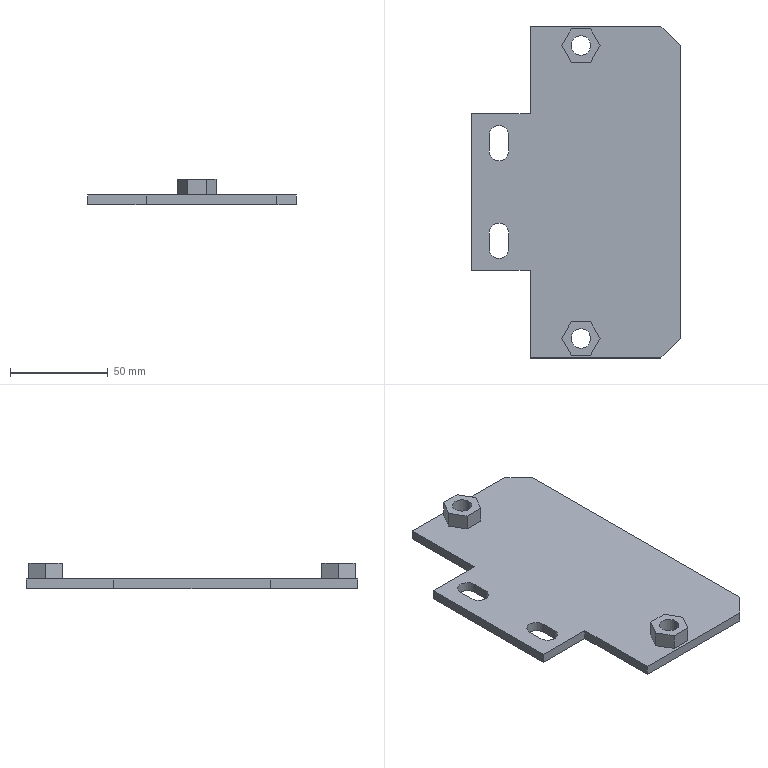Part | SolidWorks | features ICE 4, Chamfer 1, CombineBodies 1, Extrusion 1 | 3 solids | 44 faces | box 107 x 170 x 13 mm | volume 76885 mm3 | plane 32 | cylinder 12 | commonest cylinder face diameters 10 x8 12.5 x4
STEP:
#1=CARTESIAN_POINT('',(-5.,75.,13.));
#2=VERTEX_POINT('',#1);
#3=CARTESIAN_POINT('',(5.,75.,13.));
#4=VERTEX_POINT('',#3);
#5=CARTESIAN_POINT('',(0.,75.,13.));
#6=DIRECTION('',(0.,0.,1.));
#7=DIRECTION('',(1.,0.,0.));
#8=AXIS2_PLACEMENT_3D('',#5,#6,#7);
#9=CIRCLE('',#8,5.);
#10=EDGE_CURVE('',#2,#4,#9,.T.);
#11=ORIENTED_EDGE('',*,*,#10,.T.);
#12=CARTESIAN_POINT('',(5.,75.,5.));
#13=VERTEX_POINT('',#12);
#14=CARTESIAN_POINT('',(5.,75.,13.));
#15=DIRECTION('',(0.,0.,-1.));
#16=VECTOR('',#15,1000.);
#17=LINE('',#14,#16);
#18=EDGE_CURVE('',#4,#13,#17,.T.);
#19=ORIENTED_EDGE('',*,*,#18,.T.);
#20=CARTESIAN_POINT('',(-5.,75.,5.));
#21=VERTEX_POINT('',#20);
#22=CARTESIAN_POINT('',(0.,75.,5.));
#23=DIRECTION('',(0.,0.,1.));
#24=DIRECTION('',(1.,0.,0.));
#25=AXIS2_PLACEMENT_3D('',#22,#23,#24);
#26=CIRCLE('',#25,5.);
#27=EDGE_CURVE('',#21,#13,#26,.T.);
#28=ORIENTED_EDGE('',*,*,#27,.F.);
#29=CARTESIAN_POINT('',(-5.,75.,13.));
#30=DIRECTION('',(0.,0.,-1.));
#31=VECTOR('',#30,1000.);
#32=LINE('',#29,#31);
#33=EDGE_CURVE('',#2,#21,#32,.T.);
#34=ORIENTED_EDGE('',*,*,#33,.F.);
#35=EDGE_LOOP('',(#11,#19,#28,#34));
#36=FACE_OUTER_BOUND('',#35,.T.);
#37=CARTESIAN_POINT('',(0.,75.,13.));
#38=DIRECTION('',(0.,0.,-1.));
#39=DIRECTION('',(-1.,0.,0.));
#40=AXIS2_PLACEMENT_3D('',#37,#38,#39);
#41=CYLINDRICAL_SURFACE('',#40,5.);
#42=ADVANCED_FACE('',(#36),#41,.F.);
#43=CARTESIAN_POINT('',(4.907,66.5,13.));
#44=VERTEX_POINT('',#43);
#45=CARTESIAN_POINT('',(9.815,75.,13.));
#46=VERTEX_POINT('',#45);
#47=CARTESIAN_POINT('',(4.907,66.5,13.));
#48=DIRECTION('',(0.5,0.866,0.));
#49=VECTOR('',#48,1000.);
#50=LINE('',#47,#49);
#51=EDGE_CURVE('',#44,#46,#50,.T.);
#52=ORIENTED_EDGE('',*,*,#51,.T.);
#53=CARTESIAN_POINT('',(4.907,83.5,13.));
#54=VERTEX_POINT('',#53);
#55=CARTESIAN_POINT('',(9.815,75.,13.));
#56=DIRECTION('',(-0.5,0.866,0.));
#57=VECTOR('',#56,1000.);
#58=LINE('',#55,#57);
#59=EDGE_CURVE('',#46,#54,#58,.T.);
#60=ORIENTED_EDGE('',*,*,#59,.T.);
#61=CARTESIAN_POINT('',(-4.907,83.5,13.));
#62=VERTEX_POINT('',#61);
#63=CARTESIAN_POINT('',(4.907,83.5,13.));
#64=DIRECTION('',(-1.,0.,0.));
#65=VECTOR('',#64,1000.);
#66=LINE('',#63,#65);
#67=EDGE_CURVE('',#54,#62,#66,.T.);
#68=ORIENTED_EDGE('',*,*,#67,.T.);
#69=CARTESIAN_POINT('',(-9.815,75.,13.));
#70=VERTEX_POINT('',#69);
#71=CARTESIAN_POINT('',(-4.907,83.5,13.));
#72=DIRECTION('',(-0.5,-0.866,0.));
#73=VECTOR('',#72,1000.);
#74=LINE('',#71,#73);
#75=EDGE_CURVE('',#62,#70,#74,.T.);
#76=ORIENTED_EDGE('',*,*,#75,.T.);
#77=CARTESIAN_POINT('',(-4.907,66.5,13.));
#78=VERTEX_POINT('',#77);
#79=CARTESIAN_POINT('',(-9.815,75.,13.));
#80=DIRECTION('',(0.5,-0.866,0.));
#81=VECTOR('',#80,1000.);
#82=LINE('',#79,#81);
#83=EDGE_CURVE('',#70,#78,#82,.T.);
#84=ORIENTED_EDGE('',*,*,#83,.T.);
#85=CARTESIAN_POINT('',(-4.907,66.5,13.));
#86=DIRECTION('',(1.,0.,0.));
#87=VECTOR('',#86,1000.);
#88=LINE('',#85,#87);
#89=EDGE_CURVE('',#78,#44,#88,.T.);
#90=ORIENTED_EDGE('',*,*,#89,.T.);
#91=EDGE_LOOP('',(#52,#60,#68,#76,#84,#90));
#92=FACE_OUTER_BOUND('',#91,.T.);
#93=ORIENTED_EDGE('',*,*,#10,.F.);
#94=CARTESIAN_POINT('',(0.,75.,13.));
#95=DIRECTION('',(0.,0.,1.));
#96=DIRECTION('',(1.,0.,0.));
#97=AXIS2_PLACEMENT_3D('',#94,#95,#96);
#98=CIRCLE('',#97,5.);
#99=EDGE_CURVE('',#4,#2,#98,.T.);
#100=ORIENTED_EDGE('',*,*,#99,.F.);
#101=EDGE_LOOP('',(#93,#100));
#102=FACE_BOUND('',#101,.T.);
#103=CARTESIAN_POINT('',(0.,0.,13.));
#104=DIRECTION('',(0.,0.,1.));
#105=DIRECTION('',(1.,0.,0.));
#106=AXIS2_PLACEMENT_3D('',#103,#104,#105);
#107=PLANE('',#106);
#108=ADVANCED_FACE('',(#92,#102),#107,.T.);
#109=CARTESIAN_POINT('',(4.907,66.5,5.));
#110=VERTEX_POINT('',#109);
#111=CARTESIAN_POINT('',(9.815,75.,5.));
#112=VERTEX_POINT('',#111);
#113=CARTESIAN_POINT('',(4.907,66.5,5.));
#114=DIRECTION('',(0.5,0.866,0.));
#115=VECTOR('',#114,1000.);
#116=LINE('',#113,#115);
#117=EDGE_CURVE('',#110,#112,#116,.T.);
#118=ORIENTED_EDGE('',*,*,#117,.F.);
#119=CARTESIAN_POINT('',(-4.907,66.5,5.));
#120=VERTEX_POINT('',#119);
#121=CARTESIAN_POINT('',(-4.907,66.5,5.));
#122=DIRECTION('',(1.,0.,0.));
#123=VECTOR('',#122,1000.);
#124=LINE('',#121,#123);
#125=EDGE_CURVE('',#120,#110,#124,.T.);
#126=ORIENTED_EDGE('',*,*,#125,.F.);
#127=CARTESIAN_POINT('',(-9.815,75.,5.));
#128=VERTEX_POINT('',#127);
#129=CARTESIAN_POINT('',(-9.815,75.,5.));
#130=DIRECTION('',(0.5,-0.866,0.));
#131=VECTOR('',#130,1000.);
#132=LINE('',#129,#131);
#133=EDGE_CURVE('',#128,#120,#132,.T.);
#134=ORIENTED_EDGE('',*,*,#133,.F.);
#135=CARTESIAN_POINT('',(-4.907,83.5,5.));
#136=VERTEX_POINT('',#135);
#137=CARTESIAN_POINT('',(-4.907,83.5,5.));
#138=DIRECTION('',(-0.5,-0.866,0.));
#139=VECTOR('',#138,1000.);
#140=LINE('',#137,#139);
#141=EDGE_CURVE('',#136,#128,#140,.T.);
#142=ORIENTED_EDGE('',*,*,#141,.F.);
#143=CARTESIAN_POINT('',(4.907,83.5,5.));
#144=VERTEX_POINT('',#143);
#145=CARTESIAN_POINT('',(4.907,83.5,5.));
#146=DIRECTION('',(-1.,0.,0.));
#147=VECTOR('',#146,1000.);
#148=LINE('',#145,#147);
#149=EDGE_CURVE('',#144,#136,#148,.T.);
#150=ORIENTED_EDGE('',*,*,#149,.F.);
#151=CARTESIAN_POINT('',(9.815,75.,5.));
#152=DIRECTION('',(-0.5,0.866,0.));
#153=VECTOR('',#152,1000.);
#154=LINE('',#151,#153);
#155=EDGE_CURVE('',#112,#144,#154,.T.);
#156=ORIENTED_EDGE('',*,*,#155,.F.);
#157=EDGE_LOOP('',(#118,#126,#134,#142,#150,#156));
#158=FACE_OUTER_BOUND('',#157,.T.);
#159=ORIENTED_EDGE('',*,*,#27,.T.);
#160=CARTESIAN_POINT('',(0.,75.,5.));
#161=DIRECTION('',(0.,0.,1.));
#162=DIRECTION('',(1.,0.,0.));
#163=AXIS2_PLACEMENT_3D('',#160,#161,#162);
#164=CIRCLE('',#163,5.);
#165=EDGE_CURVE('',#13,#21,#164,.T.);
#166=ORIENTED_EDGE('',*,*,#165,.T.);
#167=EDGE_LOOP('',(#159,#166));
#168=FACE_BOUND('',#167,.T.);
#169=CARTESIAN_POINT('',(0.,0.,5.));
#170=DIRECTION('',(0.,0.,1.));
#171=DIRECTION('',(1.,0.,0.));
#172=AXIS2_PLACEMENT_3D('',#169,#170,#171);
#173=PLANE('',#172);
#174=ADVANCED_FACE('',(#158,#168),#173,.F.);
#175=ORIENTED_EDGE('',*,*,#117,.T.);
#176=CARTESIAN_POINT('',(9.815,75.,13.));
#177=DIRECTION('',(0.,0.,-1.));
#178=VECTOR('',#177,1000.);
#179=LINE('',#176,#178);
#180=EDGE_CURVE('',#46,#112,#179,.T.);
#181=ORIENTED_EDGE('',*,*,#180,.F.);
#182=ORIENTED_EDGE('',*,*,#51,.F.);
#183=CARTESIAN_POINT('',(4.907,66.5,13.));
#184=DIRECTION('',(0.,0.,-1.));
#185=VECTOR('',#184,1000.);
#186=LINE('',#183,#185);
#187=EDGE_CURVE('',#44,#110,#186,.T.);
#188=ORIENTED_EDGE('',*,*,#187,.T.);
#189=EDGE_LOOP('',(#175,#181,#182,#188));
#190=FACE_OUTER_BOUND('',#189,.T.);
#191=CARTESIAN_POINT('',(4.907,66.5,13.));
#192=DIRECTION('',(-0.866,0.5,0.));
#193=DIRECTION('',(-0.5,-0.866,0.));
#194=AXIS2_PLACEMENT_3D('',#191,#192,#193);
#195=PLANE('',#194);
#196=ADVANCED_FACE('',(#190),#195,.F.);
#197=ORIENTED_EDGE('',*,*,#155,.T.);
#198=CARTESIAN_POINT('',(4.907,83.5,13.));
#199=DIRECTION('',(0.,0.,-1.));
#200=VECTOR('',#199,1000.);
#201=LINE('',#198,#200);
#202=EDGE_CURVE('',#54,#144,#201,.T.);
#203=ORIENTED_EDGE('',*,*,#202,.F.);
#204=ORIENTED_EDGE('',*,*,#59,.F.);
#205=ORIENTED_EDGE('',*,*,#180,.T.);
#206=EDGE_LOOP('',(#197,#203,#204,#205));
#207=FACE_OUTER_BOUND('',#206,.T.);
#208=CARTESIAN_POINT('',(9.815,75.,13.));
#209=DIRECTION('',(-0.866,-0.5,0.));
#210=DIRECTION('',(0.5,-0.866,0.));
#211=AXIS2_PLACEMENT_3D('',#208,#209,#210);
#212=PLANE('',#211);
#213=ADVANCED_FACE('',(#207),#212,.F.);
#214=ORIENTED_EDGE('',*,*,#149,.T.);
#215=CARTESIAN_POINT('',(-4.907,83.5,13.));
#216=DIRECTION('',(0.,0.,-1.));
#217=VECTOR('',#216,1000.);
#218=LINE('',#215,#217);
#219=EDGE_CURVE('',#62,#136,#218,.T.);
#220=ORIENTED_EDGE('',*,*,#219,.F.);
#221=ORIENTED_EDGE('',*,*,#67,.F.);
#222=ORIENTED_EDGE('',*,*,#202,.T.);
#223=EDGE_LOOP('',(#214,#220,#221,#222));
#224=FACE_OUTER_BOUND('',#223,.T.);
#225=CARTESIAN_POINT('',(4.907,83.5,13.));
#226=DIRECTION('',(0.,-1.,0.));
#227=DIRECTION('',(0.,0.,-1.));
#228=AXIS2_PLACEMENT_3D('',#225,#226,#227);
#229=PLANE('',#228);
#230=ADVANCED_FACE('',(#224),#229,.F.);
#231=ORIENTED_EDGE('',*,*,#141,.T.);
#232=CARTESIAN_POINT('',(-9.815,75.,13.));
#233=DIRECTION('',(0.,0.,-1.));
#234=VECTOR('',#233,1000.);
#235=LINE('',#232,#234);
#236=EDGE_CURVE('',#70,#128,#235,.T.);
#237=ORIENTED_EDGE('',*,*,#236,.F.);
#238=ORIENTED_EDGE('',*,*,#75,.F.);
#239=ORIENTED_EDGE('',*,*,#219,.T.);
#240=EDGE_LOOP('',(#231,#237,#238,#239));
#241=FACE_OUTER_BOUND('',#240,.T.);
#242=CARTESIAN_POINT('',(-4.907,83.5,13.));
#243=DIRECTION('',(0.866,-0.5,0.));
#244=DIRECTION('',(0.5,0.866,0.));
#245=AXIS2_PLACEMENT_3D('',#242,#243,#244);
#246=PLANE('',#245);
#247=ADVANCED_FACE('',(#241),#246,.F.);
#248=ORIENTED_EDGE('',*,*,#133,.T.);
#249=CARTESIAN_POINT('',(-4.907,66.5,13.));
#250=DIRECTION('',(0.,0.,-1.));
#251=VECTOR('',#250,1000.);
#252=LINE('',#249,#251);
#253=EDGE_CURVE('',#78,#120,#252,.T.);
#254=ORIENTED_EDGE('',*,*,#253,.F.);
#255=ORIENTED_EDGE('',*,*,#83,.F.);
#256=ORIENTED_EDGE('',*,*,#236,.T.);
#257=EDGE_LOOP('',(#248,#254,#255,#256));
#258=FACE_OUTER_BOUND('',#257,.T.);
#259=CARTESIAN_POINT('',(-9.815,75.,13.));
#260=DIRECTION('',(0.866,0.5,0.));
#261=DIRECTION('',(-0.5,0.866,0.));
#262=AXIS2_PLACEMENT_3D('',#259,#260,#261);
#263=PLANE('',#262);
#264=ADVANCED_FACE('',(#258),#263,.F.);
#265=ORIENTED_EDGE('',*,*,#125,.T.);
#266=ORIENTED_EDGE('',*,*,#187,.F.);
#267=ORIENTED_EDGE('',*,*,#89,.F.);
#268=ORIENTED_EDGE('',*,*,#253,.T.);
#269=EDGE_LOOP('',(#265,#266,#267,#268));
#270=FACE_OUTER_BOUND('',#269,.T.);
#271=CARTESIAN_POINT('',(-4.907,66.5,13.));
#272=DIRECTION('',(0.,1.,0.));
#273=DIRECTION('',(-1.,0.,0.));
#274=AXIS2_PLACEMENT_3D('',#271,#272,#273);
#275=PLANE('',#274);
#276=ADVANCED_FACE('',(#270),#275,.F.);
#277=ORIENTED_EDGE('',*,*,#18,.F.);
#278=ORIENTED_EDGE('',*,*,#99,.T.);
#279=ORIENTED_EDGE('',*,*,#33,.T.);
#280=ORIENTED_EDGE('',*,*,#165,.F.);
#281=EDGE_LOOP('',(#277,#278,#279,#280));
#282=FACE_OUTER_BOUND('',#281,.T.);
#283=CARTESIAN_POINT('',(0.,75.,13.));
#284=DIRECTION('',(0.,0.,-1.));
#285=DIRECTION('',(-1.,0.,0.));
#286=AXIS2_PLACEMENT_3D('',#283,#284,#285);
#287=CYLINDRICAL_SURFACE('',#286,5.);
#288=ADVANCED_FACE('',(#282),#287,.F.);
#289=CLOSED_SHELL('',(#42,#108,#174,#196,#213,#230,#247,#264,#276,#288));
#290=MANIFOLD_SOLID_BREP('',#289);
#291=CARTESIAN_POINT('',(-5.,-75.,13.));
#292=VERTEX_POINT('',#291);
#293=CARTESIAN_POINT('',(5.,-75.,13.));
#294=VERTEX_POINT('',#293);
#295=CARTESIAN_POINT('',(0.,-75.,13.));
#296=DIRECTION('',(0.,0.,1.));
#297=DIRECTION('',(1.,0.,0.));
#298=AXIS2_PLACEMENT_3D('',#295,#296,#297);
#299=CIRCLE('',#298,5.);
#300=EDGE_CURVE('',#292,#294,#299,.T.);
#301=ORIENTED_EDGE('',*,*,#300,.T.);
#302=CARTESIAN_POINT('',(5.,-75.,5.));
#303=VERTEX_POINT('',#302);
#304=CARTESIAN_POINT('',(5.,-75.,13.));
#305=DIRECTION('',(0.,0.,-1.));
#306=VECTOR('',#305,1000.);
#307=LINE('',#304,#306);
#308=EDGE_CURVE('',#294,#303,#307,.T.);
#309=ORIENTED_EDGE('',*,*,#308,.T.);
#310=CARTESIAN_POINT('',(-5.,-75.,5.));
#311=VERTEX_POINT('',#310);
#312=CARTESIAN_POINT('',(0.,-75.,5.));
#313=DIRECTION('',(0.,0.,1.));
#314=DIRECTION('',(1.,0.,0.));
#315=AXIS2_PLACEMENT_3D('',#312,#313,#314);
#316=CIRCLE('',#315,5.);
#317=EDGE_CURVE('',#311,#303,#316,.T.);
#318=ORIENTED_EDGE('',*,*,#317,.F.);
#319=CARTESIAN_POINT('',(-5.,-75.,13.));
#320=DIRECTION('',(0.,0.,-1.));
#321=VECTOR('',#320,1000.);
#322=LINE('',#319,#321);
#323=EDGE_CURVE('',#292,#311,#322,.T.);
#324=ORIENTED_EDGE('',*,*,#323,.F.);
#325=EDGE_LOOP('',(#301,#309,#318,#324));
#326=FACE_OUTER_BOUND('',#325,.T.);
#327=CARTESIAN_POINT('',(0.,-75.,13.));
#328=DIRECTION('',(0.,0.,-1.));
#329=DIRECTION('',(-1.,0.,0.));
#330=AXIS2_PLACEMENT_3D('',#327,#328,#329);
#331=CYLINDRICAL_SURFACE('',#330,5.);
#332=ADVANCED_FACE('',(#326),#331,.F.);
#333=CARTESIAN_POINT('',(4.907,-83.5,13.));
#334=VERTEX_POINT('',#333);
#335=CARTESIAN_POINT('',(9.815,-75.,13.));
#336=VERTEX_POINT('',#335);
#337=CARTESIAN_POINT('',(4.907,-83.5,13.));
#338=DIRECTION('',(0.5,0.866,0.));
#339=VECTOR('',#338,1000.);
#340=LINE('',#337,#339);
#341=EDGE_CURVE('',#334,#336,#340,.T.);
#342=ORIENTED_EDGE('',*,*,#341,.T.);
#343=CARTESIAN_POINT('',(4.907,-66.5,13.));
#344=VERTEX_POINT('',#343);
#345=CARTESIAN_POINT('',(9.815,-75.,13.));
#346=DIRECTION('',(-0.5,0.866,0.));
#347=VECTOR('',#346,1000.);
#348=LINE('',#345,#347);
#349=EDGE_CURVE('',#336,#344,#348,.T.);
#350=ORIENTED_EDGE('',*,*,#349,.T.);
#351=CARTESIAN_POINT('',(-4.907,-66.5,13.));
#352=VERTEX_POINT('',#351);
#353=CARTESIAN_POINT('',(4.907,-66.5,13.));
#354=DIRECTION('',(-1.,0.,0.));
#355=VECTOR('',#354,1000.);
#356=LINE('',#353,#355);
#357=EDGE_CURVE('',#344,#352,#356,.T.);
#358=ORIENTED_EDGE('',*,*,#357,.T.);
#359=CARTESIAN_POINT('',(-9.815,-75.,13.));
#360=VERTEX_POINT('',#359);
#361=CARTESIAN_POINT('',(-4.907,-66.5,13.));
#362=DIRECTION('',(-0.5,-0.866,0.));
#363=VECTOR('',#362,1000.);
#364=LINE('',#361,#363);
#365=EDGE_CURVE('',#352,#360,#364,.T.);
#366=ORIENTED_EDGE('',*,*,#365,.T.);
#367=CARTESIAN_POINT('',(-4.907,-83.5,13.));
#368=VERTEX_POINT('',#367);
#369=CARTESIAN_POINT('',(-9.815,-75.,13.));
#370=DIRECTION('',(0.5,-0.866,0.));
#371=VECTOR('',#370,1000.);
#372=LINE('',#369,#371);
#373=EDGE_CURVE('',#360,#368,#372,.T.);
#374=ORIENTED_EDGE('',*,*,#373,.T.);
#375=CARTESIAN_POINT('',(-4.907,-83.5,13.));
#376=DIRECTION('',(1.,0.,0.));
#377=VECTOR('',#376,1000.);
#378=LINE('',#375,#377);
#379=EDGE_CURVE('',#368,#334,#378,.T.);
#380=ORIENTED_EDGE('',*,*,#379,.T.);
#381=EDGE_LOOP('',(#342,#350,#358,#366,#374,#380));
#382=FACE_OUTER_BOUND('',#381,.T.);
#383=ORIENTED_EDGE('',*,*,#300,.F.);
#384=CARTESIAN_POINT('',(0.,-75.,13.));
#385=DIRECTION('',(0.,0.,1.));
#386=DIRECTION('',(1.,0.,0.));
#387=AXIS2_PLACEMENT_3D('',#384,#385,#386);
#388=CIRCLE('',#387,5.);
#389=EDGE_CURVE('',#294,#292,#388,.T.);
#390=ORIENTED_EDGE('',*,*,#389,.F.);
#391=EDGE_LOOP('',(#383,#390));
#392=FACE_BOUND('',#391,.T.);
#393=CARTESIAN_POINT('',(0.,0.,13.));
#394=DIRECTION('',(0.,0.,1.));
#395=DIRECTION('',(1.,0.,0.));
#396=AXIS2_PLACEMENT_3D('',#393,#394,#395);
#397=PLANE('',#396);
#398=ADVANCED_FACE('',(#382,#392),#397,.T.);
#399=CARTESIAN_POINT('',(4.907,-83.5,5.));
#400=VERTEX_POINT('',#399);
#401=CARTESIAN_POINT('',(9.815,-75.,5.));
#402=VERTEX_POINT('',#401);
#403=CARTESIAN_POINT('',(4.907,-83.5,5.));
#404=DIRECTION('',(0.5,0.866,0.));
#405=VECTOR('',#404,1000.);
#406=LINE('',#403,#405);
#407=EDGE_CURVE('',#400,#402,#406,.T.);
#408=ORIENTED_EDGE('',*,*,#407,.F.);
#409=CARTESIAN_POINT('',(-4.907,-83.5,5.));
#410=VERTEX_POINT('',#409);
#411=CARTESIAN_POINT('',(-4.907,-83.5,5.));
#412=DIRECTION('',(1.,0.,0.));
#413=VECTOR('',#412,1000.);
#414=LINE('',#411,#413);
#415=EDGE_CURVE('',#410,#400,#414,.T.);
#416=ORIENTED_EDGE('',*,*,#415,.F.);
#417=CARTESIAN_POINT('',(-9.815,-75.,5.));
#418=VERTEX_POINT('',#417);
#419=CARTESIAN_POINT('',(-9.815,-75.,5.));
#420=DIRECTION('',(0.5,-0.866,0.));
#421=VECTOR('',#420,1000.);
#422=LINE('',#419,#421);
#423=EDGE_CURVE('',#418,#410,#422,.T.);
#424=ORIENTED_EDGE('',*,*,#423,.F.);
#425=CARTESIAN_POINT('',(-4.907,-66.5,5.));
#426=VERTEX_POINT('',#425);
#427=CARTESIAN_POINT('',(-4.907,-66.5,5.));
#428=DIRECTION('',(-0.5,-0.866,0.));
#429=VECTOR('',#428,1000.);
#430=LINE('',#427,#429);
#431=EDGE_CURVE('',#426,#418,#430,.T.);
#432=ORIENTED_EDGE('',*,*,#431,.F.);
#433=CARTESIAN_POINT('',(4.907,-66.5,5.));
#434=VERTEX_POINT('',#433);
#435=CARTESIAN_POINT('',(4.907,-66.5,5.));
#436=DIRECTION('',(-1.,0.,0.));
#437=VECTOR('',#436,1000.);
#438=LINE('',#435,#437);
#439=EDGE_CURVE('',#434,#426,#438,.T.);
#440=ORIENTED_EDGE('',*,*,#439,.F.);
#441=CARTESIAN_POINT('',(9.815,-75.,5.));
#442=DIRECTION('',(-0.5,0.866,0.));
#443=VECTOR('',#442,1000.);
#444=LINE('',#441,#443);
#445=EDGE_CURVE('',#402,#434,#444,.T.);
#446=ORIENTED_EDGE('',*,*,#445,.F.);
#447=EDGE_LOOP('',(#408,#416,#424,#432,#440,#446));
#448=FACE_OUTER_BOUND('',#447,.T.);
#449=ORIENTED_EDGE('',*,*,#317,.T.);
#450=CARTESIAN_POINT('',(0.,-75.,5.));
#451=DIRECTION('',(0.,0.,1.));
#452=DIRECTION('',(1.,0.,0.));
#453=AXIS2_PLACEMENT_3D('',#450,#451,#452);
#454=CIRCLE('',#453,5.);
#455=EDGE_CURVE('',#303,#311,#454,.T.);
#456=ORIENTED_EDGE('',*,*,#455,.T.);
#457=EDGE_LOOP('',(#449,#456));
#458=FACE_BOUND('',#457,.T.);
#459=CARTESIAN_POINT('',(0.,0.,5.));
#460=DIRECTION('',(0.,0.,1.));
#461=DIRECTION('',(1.,0.,0.));
#462=AXIS2_PLACEMENT_3D('',#459,#460,#461);
#463=PLANE('',#462);
#464=ADVANCED_FACE('',(#448,#458),#463,.F.);
#465=ORIENTED_EDGE('',*,*,#407,.T.);
#466=CARTESIAN_POINT('',(9.815,-75.,13.));
#467=DIRECTION('',(0.,0.,-1.));
#468=VECTOR('',#467,1000.);
#469=LINE('',#466,#468);
#470=EDGE_CURVE('',#336,#402,#469,.T.);
#471=ORIENTED_EDGE('',*,*,#470,.F.);
#472=ORIENTED_EDGE('',*,*,#341,.F.);
#473=CARTESIAN_POINT('',(4.907,-83.5,13.));
#474=DIRECTION('',(0.,0.,-1.));
#475=VECTOR('',#474,1000.);
#476=LINE('',#473,#475);
#477=EDGE_CURVE('',#334,#400,#476,.T.);
#478=ORIENTED_EDGE('',*,*,#477,.T.);
#479=EDGE_LOOP('',(#465,#471,#472,#478));
#480=FACE_OUTER_BOUND('',#479,.T.);
#481=CARTESIAN_POINT('',(4.907,-83.5,13.));
#482=DIRECTION('',(-0.866,0.5,0.));
#483=DIRECTION('',(-0.5,-0.866,0.));
#484=AXIS2_PLACEMENT_3D('',#481,#482,#483);
#485=PLANE('',#484);
#486=ADVANCED_FACE('',(#480),#485,.F.);
#487=ORIENTED_EDGE('',*,*,#445,.T.);
#488=CARTESIAN_POINT('',(4.907,-66.5,13.));
#489=DIRECTION('',(0.,0.,-1.));
#490=VECTOR('',#489,1000.);
#491=LINE('',#488,#490);
#492=EDGE_CURVE('',#344,#434,#491,.T.);
#493=ORIENTED_EDGE('',*,*,#492,.F.);
#494=ORIENTED_EDGE('',*,*,#349,.F.);
#495=ORIENTED_EDGE('',*,*,#470,.T.);
#496=EDGE_LOOP('',(#487,#493,#494,#495));
#497=FACE_OUTER_BOUND('',#496,.T.);
#498=CARTESIAN_POINT('',(9.815,-75.,13.));
#499=DIRECTION('',(-0.866,-0.5,0.));
#500=DIRECTION('',(0.5,-0.866,0.));
#501=AXIS2_PLACEMENT_3D('',#498,#499,#500);
#502=PLANE('',#501);
#503=ADVANCED_FACE('',(#497),#502,.F.);
#504=ORIENTED_EDGE('',*,*,#439,.T.);
#505=CARTESIAN_POINT('',(-4.907,-66.5,13.));
#506=DIRECTION('',(0.,0.,-1.));
#507=VECTOR('',#506,1000.);
#508=LINE('',#505,#507);
#509=EDGE_CURVE('',#352,#426,#508,.T.);
#510=ORIENTED_EDGE('',*,*,#509,.F.);
#511=ORIENTED_EDGE('',*,*,#357,.F.);
#512=ORIENTED_EDGE('',*,*,#492,.T.);
#513=EDGE_LOOP('',(#504,#510,#511,#512));
#514=FACE_OUTER_BOUND('',#513,.T.);
#515=CARTESIAN_POINT('',(4.907,-66.5,13.));
#516=DIRECTION('',(0.,-1.,0.));
#517=DIRECTION('',(1.,0.,0.));
#518=AXIS2_PLACEMENT_3D('',#515,#516,#517);
#519=PLANE('',#518);
#520=ADVANCED_FACE('',(#514),#519,.F.);
#521=ORIENTED_EDGE('',*,*,#431,.T.);
#522=CARTESIAN_POINT('',(-9.815,-75.,13.));
#523=DIRECTION('',(0.,0.,-1.));
#524=VECTOR('',#523,1000.);
#525=LINE('',#522,#524);
#526=EDGE_CURVE('',#360,#418,#525,.T.);
#527=ORIENTED_EDGE('',*,*,#526,.F.);
#528=ORIENTED_EDGE('',*,*,#365,.F.);
#529=ORIENTED_EDGE('',*,*,#509,.T.);
#530=EDGE_LOOP('',(#521,#527,#528,#529));
#531=FACE_OUTER_BOUND('',#530,.T.);
#532=CARTESIAN_POINT('',(-4.907,-66.5,13.));
#533=DIRECTION('',(0.866,-0.5,0.));
#534=DIRECTION('',(0.5,0.866,0.));
#535=AXIS2_PLACEMENT_3D('',#532,#533,#534);
#536=PLANE('',#535);
#537=ADVANCED_FACE('',(#531),#536,.F.);
#538=ORIENTED_EDGE('',*,*,#423,.T.);
#539=CARTESIAN_POINT('',(-4.907,-83.5,13.));
#540=DIRECTION('',(0.,0.,-1.));
#541=VECTOR('',#540,1000.);
#542=LINE('',#539,#541);
#543=EDGE_CURVE('',#368,#410,#542,.T.);
#544=ORIENTED_EDGE('',*,*,#543,.F.);
#545=ORIENTED_EDGE('',*,*,#373,.F.);
#546=ORIENTED_EDGE('',*,*,#526,.T.);
#547=EDGE_LOOP('',(#538,#544,#545,#546));
#548=FACE_OUTER_BOUND('',#547,.T.);
#549=CARTESIAN_POINT('',(-9.815,-75.,13.));
#550=DIRECTION('',(0.866,0.5,0.));
#551=DIRECTION('',(-0.5,0.866,0.));
#552=AXIS2_PLACEMENT_3D('',#549,#550,#551);
#553=PLANE('',#552);
#554=ADVANCED_FACE('',(#548),#553,.F.);
#555=ORIENTED_EDGE('',*,*,#415,.T.);
#556=ORIENTED_EDGE('',*,*,#477,.F.);
#557=ORIENTED_EDGE('',*,*,#379,.F.);
#558=ORIENTED_EDGE('',*,*,#543,.T.);
#559=EDGE_LOOP('',(#555,#556,#557,#558));
#560=FACE_OUTER_BOUND('',#559,.T.);
#561=CARTESIAN_POINT('',(-4.907,-83.5,13.));
#562=DIRECTION('',(0.,1.,0.));
#563=DIRECTION('',(-1.,0.,0.));
#564=AXIS2_PLACEMENT_3D('',#561,#562,#563);
#565=PLANE('',#564);
#566=ADVANCED_FACE('',(#560),#565,.F.);
#567=ORIENTED_EDGE('',*,*,#308,.F.);
#568=ORIENTED_EDGE('',*,*,#389,.T.);
#569=ORIENTED_EDGE('',*,*,#323,.T.);
#570=ORIENTED_EDGE('',*,*,#455,.F.);
#571=EDGE_LOOP('',(#567,#568,#569,#570));
#572=FACE_OUTER_BOUND('',#571,.T.);
#573=CARTESIAN_POINT('',(0.,-75.,13.));
#574=DIRECTION('',(0.,0.,-1.));
#575=DIRECTION('',(-1.,0.,0.));
#576=AXIS2_PLACEMENT_3D('',#573,#574,#575);
#577=CYLINDRICAL_SURFACE('',#576,5.);
#578=ADVANCED_FACE('',(#572),#577,.F.);
#579=CLOSED_SHELL('',(#332,#398,#464,#486,#503,#520,#537,#554,#566,#578));
#580=MANIFOLD_SOLID_BREP('',#579);
#581=CARTESIAN_POINT('',(-6.25,-75.,5.));
#582=VERTEX_POINT('',#581);
#583=CARTESIAN_POINT('',(6.25,-75.,5.));
#584=VERTEX_POINT('',#583);
#585=CARTESIAN_POINT('',(0.,-75.,5.));
#586=DIRECTION('',(0.,0.,1.));
#587=DIRECTION('',(1.,0.,0.));
#588=AXIS2_PLACEMENT_3D('',#585,#586,#587);
#589=CIRCLE('',#588,6.25);
#590=EDGE_CURVE('',#582,#584,#589,.T.);
#591=ORIENTED_EDGE('',*,*,#590,.T.);
#592=CARTESIAN_POINT('',(6.25,-75.,0.));
#593=VERTEX_POINT('',#592);
#594=CARTESIAN_POINT('',(6.25,-75.,5.));
#595=DIRECTION('',(0.,0.,-1.));
#596=VECTOR('',#595,1000.);
#597=LINE('',#594,#596);
#598=EDGE_CURVE('',#584,#593,#597,.T.);
#599=ORIENTED_EDGE('',*,*,#598,.T.);
#600=CARTESIAN_POINT('',(-6.25,-75.,0.));
#601=VERTEX_POINT('',#600);
#602=CARTESIAN_POINT('',(0.,-75.,0.));
#603=DIRECTION('',(0.,0.,1.));
#604=DIRECTION('',(1.,0.,0.));
#605=AXIS2_PLACEMENT_3D('',#602,#603,#604);
#606=CIRCLE('',#605,6.25);
#607=EDGE_CURVE('',#601,#593,#606,.T.);
#608=ORIENTED_EDGE('',*,*,#607,.F.);
#609=CARTESIAN_POINT('',(-6.25,-75.,5.));
#610=DIRECTION('',(0.,0.,-1.));
#611=VECTOR('',#610,1000.);
#612=LINE('',#609,#611);
#613=EDGE_CURVE('',#582,#601,#612,.T.);
#614=ORIENTED_EDGE('',*,*,#613,.F.);
#615=EDGE_LOOP('',(#591,#599,#608,#614));
#616=FACE_OUTER_BOUND('',#615,.T.);
#617=CARTESIAN_POINT('',(0.,-75.,5.));
#618=DIRECTION('',(0.,0.,-1.));
#619=DIRECTION('',(-1.,0.,0.));
#620=AXIS2_PLACEMENT_3D('',#617,#618,#619);
#621=CYLINDRICAL_SURFACE('',#620,6.25);
#622=ADVANCED_FACE('',(#616),#621,.F.);
#623=CARTESIAN_POINT('',(-6.25,75.,5.));
#624=VERTEX_POINT('',#623);
#625=CARTESIAN_POINT('',(6.25,75.,5.));
#626=VERTEX_POINT('',#625);
#627=CARTESIAN_POINT('',(0.,75.,5.));
#628=DIRECTION('',(0.,0.,1.));
#629=DIRECTION('',(1.,0.,0.));
#630=AXIS2_PLACEMENT_3D('',#627,#628,#629);
#631=CIRCLE('',#630,6.25);
#632=EDGE_CURVE('',#624,#626,#631,.T.);
#633=ORIENTED_EDGE('',*,*,#632,.T.);
#634=CARTESIAN_POINT('',(6.25,75.,0.));
#635=VERTEX_POINT('',#634);
#636=CARTESIAN_POINT('',(6.25,75.,5.));
#637=DIRECTION('',(0.,0.,-1.));
#638=VECTOR('',#637,1000.);
#639=LINE('',#636,#638);
#640=EDGE_CURVE('',#626,#635,#639,.T.);
#641=ORIENTED_EDGE('',*,*,#640,.T.);
#642=CARTESIAN_POINT('',(-6.25,75.,0.));
#643=VERTEX_POINT('',#642);
#644=CARTESIAN_POINT('',(0.,75.,0.));
#645=DIRECTION('',(0.,0.,1.));
#646=DIRECTION('',(1.,0.,0.));
#647=AXIS2_PLACEMENT_3D('',#644,#645,#646);
#648=CIRCLE('',#647,6.25);
#649=EDGE_CURVE('',#643,#635,#648,.T.);
#650=ORIENTED_EDGE('',*,*,#649,.F.);
#651=CARTESIAN_POINT('',(-6.25,75.,5.));
#652=DIRECTION('',(0.,0.,-1.));
#653=VECTOR('',#652,1000.);
#654=LINE('',#651,#653);
#655=EDGE_CURVE('',#624,#643,#654,.T.);
#656=ORIENTED_EDGE('',*,*,#655,.F.);
#657=EDGE_LOOP('',(#633,#641,#650,#656));
#658=FACE_OUTER_BOUND('',#657,.T.);
#659=CARTESIAN_POINT('',(0.,75.,5.));
#660=DIRECTION('',(0.,0.,-1.));
#661=DIRECTION('',(-1.,0.,0.));
#662=AXIS2_PLACEMENT_3D('',#659,#660,#661);
#663=CYLINDRICAL_SURFACE('',#662,6.25);
#664=ADVANCED_FACE('',(#658),#663,.F.);
#665=CARTESIAN_POINT('',(-26.,40.,5.));
#666=VERTEX_POINT('',#665);
#667=CARTESIAN_POINT('',(-26.,40.,0.));
#668=VERTEX_POINT('',#667);
#669=CARTESIAN_POINT('',(-26.,40.,90.44));
#670=DIRECTION('',(0.,0.,-1.));
#671=VECTOR('',#670,1000.);
#672=LINE('',#669,#671);
#673=EDGE_CURVE('',#666,#668,#672,.T.);
#674=ORIENTED_EDGE('',*,*,#673,.F.);
#675=CARTESIAN_POINT('',(-26.,85.,5.));
#676=VERTEX_POINT('',#675);
#677=CARTESIAN_POINT('',(-26.,85.,5.));
#678=DIRECTION('',(0.,-1.,0.));
#679=VECTOR('',#678,1000.);
#680=LINE('',#677,#679);
#681=EDGE_CURVE('',#676,#666,#680,.T.);
#682=ORIENTED_EDGE('',*,*,#681,.F.);
#683=CARTESIAN_POINT('',(-26.,85.,0.));
#684=VERTEX_POINT('',#683);
#685=CARTESIAN_POINT('',(-26.,85.,5.));
#686=DIRECTION('',(0.,0.,-1.));
#687=VECTOR('',#686,1000.);
#688=LINE('',#685,#687);
#689=EDGE_CURVE('',#676,#684,#688,.T.);
#690=ORIENTED_EDGE('',*,*,#689,.T.);
#691=CARTESIAN_POINT('',(-26.,85.,0.));
#692=DIRECTION('',(0.,-1.,0.));
#693=VECTOR('',#692,1000.);
#694=LINE('',#691,#693);
#695=EDGE_CURVE('',#684,#668,#694,.T.);
#696=ORIENTED_EDGE('',*,*,#695,.T.);
#697=EDGE_LOOP('',(#674,#682,#690,#696));
#698=FACE_OUTER_BOUND('',#697,.T.);
#699=CARTESIAN_POINT('',(-26.,85.,5.));
#700=DIRECTION('',(1.,0.,0.));
#701=DIRECTION('',(0.,1.,0.));
#702=AXIS2_PLACEMENT_3D('',#699,#700,#701);
#703=PLANE('',#702);
#704=ADVANCED_FACE('',(#698),#703,.F.);
#705=CARTESIAN_POINT('',(-47.,-29.,5.));
#706=VERTEX_POINT('',#705);
#707=CARTESIAN_POINT('',(-37.,-29.,5.));
#708=VERTEX_POINT('',#707);
#709=CARTESIAN_POINT('',(-42.,-29.,5.));
#710=DIRECTION('',(0.,0.,1.));
#711=DIRECTION('',(1.,0.,0.));
#712=AXIS2_PLACEMENT_3D('',#709,#710,#711);
#713=CIRCLE('',#712,5.);
#714=EDGE_CURVE('',#706,#708,#713,.T.);
#715=ORIENTED_EDGE('',*,*,#714,.F.);
#716=CARTESIAN_POINT('',(-47.,-21.,5.));
#717=VERTEX_POINT('',#716);
#718=CARTESIAN_POINT('',(-47.,-29.,5.));
#719=DIRECTION('',(0.,-1.,0.));
#720=VECTOR('',#719,1000.);
#721=LINE('',#718,#720);
#722=EDGE_CURVE('',#717,#706,#721,.T.);
#723=ORIENTED_EDGE('',*,*,#722,.F.);
#724=CARTESIAN_POINT('',(-37.,-21.,5.));
#725=VERTEX_POINT('',#724);
#726=CARTESIAN_POINT('',(-42.,-21.,5.));
#727=DIRECTION('',(0.,0.,1.));
#728=DIRECTION('',(1.,0.,0.));
#729=AXIS2_PLACEMENT_3D('',#726,#727,#728);
#730=CIRCLE('',#729,5.);
#731=EDGE_CURVE('',#725,#717,#730,.T.);
#732=ORIENTED_EDGE('',*,*,#731,.F.);
#733=CARTESIAN_POINT('',(-37.,-29.,5.));
#734=DIRECTION('',(0.,1.,0.));
#735=VECTOR('',#734,1000.);
#736=LINE('',#733,#735);
#737=EDGE_CURVE('',#708,#725,#736,.T.);
#738=ORIENTED_EDGE('',*,*,#737,.F.);
#739=EDGE_LOOP('',(#715,#723,#732,#738));
#740=FACE_BOUND('',#739,.T.);
#741=CARTESIAN_POINT('',(-37.,29.,5.));
#742=VERTEX_POINT('',#741);
#743=CARTESIAN_POINT('',(-47.,29.,5.));
#744=VERTEX_POINT('',#743);
#745=CARTESIAN_POINT('',(-42.,29.,5.));
#746=DIRECTION('',(0.,0.,1.));
#747=DIRECTION('',(-1.,0.,0.));
#748=AXIS2_PLACEMENT_3D('',#745,#746,#747);
#749=CIRCLE('',#748,5.);
#750=EDGE_CURVE('',#742,#744,#749,.T.);
#751=ORIENTED_EDGE('',*,*,#750,.F.);
#752=CARTESIAN_POINT('',(-37.,21.,5.));
#753=VERTEX_POINT('',#752);
#754=CARTESIAN_POINT('',(-37.,29.,5.));
#755=DIRECTION('',(0.,1.,0.));
#756=VECTOR('',#755,1000.);
#757=LINE('',#754,#756);
#758=EDGE_CURVE('',#753,#742,#757,.T.);
#759=ORIENTED_EDGE('',*,*,#758,.F.);
#760=CARTESIAN_POINT('',(-47.,21.,5.));
#761=VERTEX_POINT('',#760);
#762=CARTESIAN_POINT('',(-42.,21.,5.));
#763=DIRECTION('',(0.,0.,1.));
#764=DIRECTION('',(-1.,0.,0.));
#765=AXIS2_PLACEMENT_3D('',#762,#763,#764);
#766=CIRCLE('',#765,5.);
#767=EDGE_CURVE('',#761,#753,#766,.T.);
#768=ORIENTED_EDGE('',*,*,#767,.F.);
#769=CARTESIAN_POINT('',(-47.,29.,5.));
#770=DIRECTION('',(0.,-1.,0.));
#771=VECTOR('',#770,1000.);
#772=LINE('',#769,#771);
#773=EDGE_CURVE('',#744,#761,#772,.T.);
#774=ORIENTED_EDGE('',*,*,#773,.F.);
#775=EDGE_LOOP('',(#751,#759,#768,#774));
#776=FACE_BOUND('',#775,.T.);
#777=ORIENTED_EDGE('',*,*,#632,.F.);
#778=CARTESIAN_POINT('',(0.,75.,5.));
#779=DIRECTION('',(0.,0.,1.));
#780=DIRECTION('',(1.,0.,0.));
#781=AXIS2_PLACEMENT_3D('',#778,#779,#780);
#782=CIRCLE('',#781,6.25);
#783=EDGE_CURVE('',#626,#624,#782,.T.);
#784=ORIENTED_EDGE('',*,*,#783,.F.);
#785=EDGE_LOOP('',(#777,#784));
#786=FACE_BOUND('',#785,.T.);
#787=CARTESIAN_POINT('',(51.,-75.,5.));
#788=VERTEX_POINT('',#787);
#789=CARTESIAN_POINT('',(51.,75.,5.));
#790=VERTEX_POINT('',#789);
#791=CARTESIAN_POINT('',(51.,-85.,5.));
#792=DIRECTION('',(0.,1.,0.));
#793=VECTOR('',#792,1000.);
#794=LINE('',#791,#793);
#795=EDGE_CURVE('',#788,#790,#794,.T.);
#796=ORIENTED_EDGE('',*,*,#795,.T.);
#797=CARTESIAN_POINT('',(41.,85.,5.));
#798=VERTEX_POINT('',#797);
#799=CARTESIAN_POINT('',(63.,63.,5.));
#800=DIRECTION('',(-0.7071,0.7071,0.));
#801=VECTOR('',#800,1000.);
#802=LINE('',#799,#801);
#803=EDGE_CURVE('',#790,#798,#802,.T.);
#804=ORIENTED_EDGE('',*,*,#803,.T.);
#805=CARTESIAN_POINT('',(-26.,85.,5.));
#806=DIRECTION('',(-1.,0.,0.));
#807=VECTOR('',#806,1000.);
#808=LINE('',#805,#807);
#809=EDGE_CURVE('',#798,#676,#808,.T.);
#810=ORIENTED_EDGE('',*,*,#809,.T.);
#811=ORIENTED_EDGE('',*,*,#681,.T.);
#812=CARTESIAN_POINT('',(-56.,40.,5.));
#813=VERTEX_POINT('',#812);
#814=CARTESIAN_POINT('',(-26.,40.,5.));
#815=DIRECTION('',(1.,0.,0.));
#816=VECTOR('',#815,1000.);
#817=LINE('',#814,#816);
#818=EDGE_CURVE('',#813,#666,#817,.T.);
#819=ORIENTED_EDGE('',*,*,#818,.F.);
#820=CARTESIAN_POINT('',(-56.,-40.,5.));
#821=VERTEX_POINT('',#820);
#822=CARTESIAN_POINT('',(-56.,40.,5.));
#823=DIRECTION('',(0.,1.,0.));
#824=VECTOR('',#823,1000.);
#825=LINE('',#822,#824);
#826=EDGE_CURVE('',#821,#813,#825,.T.);
#827=ORIENTED_EDGE('',*,*,#826,.F.);
#828=CARTESIAN_POINT('',(-26.,-40.,5.));
#829=VERTEX_POINT('',#828);
#830=CARTESIAN_POINT('',(-26.,-40.,5.));
#831=DIRECTION('',(-1.,0.,0.));
#832=VECTOR('',#831,1000.);
#833=LINE('',#830,#832);
#834=EDGE_CURVE('',#829,#821,#833,.T.);
#835=ORIENTED_EDGE('',*,*,#834,.F.);
#836=CARTESIAN_POINT('',(-26.,-85.,5.));
#837=VERTEX_POINT('',#836);
#838=CARTESIAN_POINT('',(-26.,85.,5.));
#839=DIRECTION('',(0.,-1.,0.));
#840=VECTOR('',#839,1000.);
#841=LINE('',#838,#840);
#842=EDGE_CURVE('',#829,#837,#841,.T.);
#843=ORIENTED_EDGE('',*,*,#842,.T.);
#844=CARTESIAN_POINT('',(41.,-85.,5.));
#845=VERTEX_POINT('',#844);
#846=CARTESIAN_POINT('',(-26.,-85.,5.));
#847=DIRECTION('',(1.,0.,0.));
#848=VECTOR('',#847,1000.);
#849=LINE('',#846,#848);
#850=EDGE_CURVE('',#837,#845,#849,.T.);
#851=ORIENTED_EDGE('',*,*,#850,.T.);
#852=CARTESIAN_POINT('',(63.,-63.,5.));
#853=DIRECTION('',(0.7071,0.7071,0.));
#854=VECTOR('',#853,1000.);
#855=LINE('',#852,#854);
#856=EDGE_CURVE('',#845,#788,#855,.T.);
#857=ORIENTED_EDGE('',*,*,#856,.T.);
#858=EDGE_LOOP('',(#796,#804,#810,#811,#819,#827,#835,#843,#851,#857));
#859=FACE_OUTER_BOUND('',#858,.T.);
#860=ORIENTED_EDGE('',*,*,#590,.F.);
#861=CARTESIAN_POINT('',(0.,-75.,5.));
#862=DIRECTION('',(0.,0.,1.));
#863=DIRECTION('',(1.,0.,0.));
#864=AXIS2_PLACEMENT_3D('',#861,#862,#863);
#865=CIRCLE('',#864,6.25);
#866=EDGE_CURVE('',#584,#582,#865,.T.);
#867=ORIENTED_EDGE('',*,*,#866,.F.);
#868=EDGE_LOOP('',(#860,#867));
#869=FACE_BOUND('',#868,.T.);
#870=CARTESIAN_POINT('',(0.,0.,5.));
#871=DIRECTION('',(0.,0.,1.));
#872=DIRECTION('',(1.,0.,0.));
#873=AXIS2_PLACEMENT_3D('',#870,#871,#872);
#874=PLANE('',#873);
#875=ADVANCED_FACE('',(#740,#776,#786,#859,#869),#874,.T.);
#876=CARTESIAN_POINT('',(-47.,-21.,0.));
#877=VERTEX_POINT('',#876);
#878=CARTESIAN_POINT('',(-47.,-29.,0.));
#879=VERTEX_POINT('',#878);
#880=CARTESIAN_POINT('',(-47.,-29.,0.));
#881=DIRECTION('',(0.,-1.,0.));
#882=VECTOR('',#881,1000.);
#883=LINE('',#880,#882);
#884=EDGE_CURVE('',#877,#879,#883,.T.);
#885=ORIENTED_EDGE('',*,*,#884,.T.);
#886=CARTESIAN_POINT('',(-37.,-29.,0.));
#887=VERTEX_POINT('',#886);
#888=CARTESIAN_POINT('',(-42.,-29.,0.));
#889=DIRECTION('',(0.,0.,1.));
#890=DIRECTION('',(1.,0.,0.));
#891=AXIS2_PLACEMENT_3D('',#888,#889,#890);
#892=CIRCLE('',#891,5.);
#893=EDGE_CURVE('',#879,#887,#892,.T.);
#894=ORIENTED_EDGE('',*,*,#893,.T.);
#895=CARTESIAN_POINT('',(-37.,-21.,0.));
#896=VERTEX_POINT('',#895);
#897=CARTESIAN_POINT('',(-37.,-29.,0.));
#898=DIRECTION('',(0.,1.,0.));
#899=VECTOR('',#898,1000.);
#900=LINE('',#897,#899);
#901=EDGE_CURVE('',#887,#896,#900,.T.);
#902=ORIENTED_EDGE('',*,*,#901,.T.);
#903=CARTESIAN_POINT('',(-42.,-21.,0.));
#904=DIRECTION('',(0.,0.,1.));
#905=DIRECTION('',(1.,0.,0.));
#906=AXIS2_PLACEMENT_3D('',#903,#904,#905);
#907=CIRCLE('',#906,5.);
#908=EDGE_CURVE('',#896,#877,#907,.T.);
#909=ORIENTED_EDGE('',*,*,#908,.T.);
#910=EDGE_LOOP('',(#885,#894,#902,#909));
#911=FACE_BOUND('',#910,.T.);
#912=CARTESIAN_POINT('',(-37.,21.,0.));
#913=VERTEX_POINT('',#912);
#914=CARTESIAN_POINT('',(-37.,29.,0.));
#915=VERTEX_POINT('',#914);
#916=CARTESIAN_POINT('',(-37.,29.,0.));
#917=DIRECTION('',(0.,1.,0.));
#918=VECTOR('',#917,1000.);
#919=LINE('',#916,#918);
#920=EDGE_CURVE('',#913,#915,#919,.T.);
#921=ORIENTED_EDGE('',*,*,#920,.T.);
#922=CARTESIAN_POINT('',(-47.,29.,0.));
#923=VERTEX_POINT('',#922);
#924=CARTESIAN_POINT('',(-42.,29.,0.));
#925=DIRECTION('',(0.,0.,1.));
#926=DIRECTION('',(-1.,0.,0.));
#927=AXIS2_PLACEMENT_3D('',#924,#925,#926);
#928=CIRCLE('',#927,5.);
#929=EDGE_CURVE('',#915,#923,#928,.T.);
#930=ORIENTED_EDGE('',*,*,#929,.T.);
#931=CARTESIAN_POINT('',(-47.,21.,0.));
#932=VERTEX_POINT('',#931);
#933=CARTESIAN_POINT('',(-47.,29.,0.));
#934=DIRECTION('',(0.,-1.,0.));
#935=VECTOR('',#934,1000.);
#936=LINE('',#933,#935);
#937=EDGE_CURVE('',#923,#932,#936,.T.);
#938=ORIENTED_EDGE('',*,*,#937,.T.);
#939=CARTESIAN_POINT('',(-42.,21.,0.));
#940=DIRECTION('',(0.,0.,1.));
#941=DIRECTION('',(-1.,0.,0.));
#942=AXIS2_PLACEMENT_3D('',#939,#940,#941);
#943=CIRCLE('',#942,5.);
#944=EDGE_CURVE('',#932,#913,#943,.T.);
#945=ORIENTED_EDGE('',*,*,#944,.T.);
#946=EDGE_LOOP('',(#921,#930,#938,#945));
#947=FACE_BOUND('',#946,.T.);
#948=CARTESIAN_POINT('',(41.,85.,0.));
#949=VERTEX_POINT('',#948);
#950=CARTESIAN_POINT('',(-26.,85.,0.));
#951=DIRECTION('',(-1.,0.,0.));
#952=VECTOR('',#951,1000.);
#953=LINE('',#950,#952);
#954=EDGE_CURVE('',#949,#684,#953,.T.);
#955=ORIENTED_EDGE('',*,*,#954,.F.);
#956=CARTESIAN_POINT('',(51.,75.,0.));
#957=VERTEX_POINT('',#956);
#958=CARTESIAN_POINT('',(51.,75.,0.));
#959=DIRECTION('',(0.7071,-0.7071,0.));
#960=VECTOR('',#959,1000.);
#961=LINE('',#958,#960);
#962=EDGE_CURVE('',#949,#957,#961,.T.);
#963=ORIENTED_EDGE('',*,*,#962,.T.);
#964=CARTESIAN_POINT('',(51.,-75.,0.));
#965=VERTEX_POINT('',#964);
#966=CARTESIAN_POINT('',(51.,-85.,0.));
#967=DIRECTION('',(0.,-1.,0.));
#968=VECTOR('',#967,1000.);
#969=LINE('',#966,#968);
#970=EDGE_CURVE('',#957,#965,#969,.T.);
#971=ORIENTED_EDGE('',*,*,#970,.T.);
#972=CARTESIAN_POINT('',(41.,-85.,0.));
#973=VERTEX_POINT('',#972);
#974=CARTESIAN_POINT('',(41.,-85.,0.));
#975=DIRECTION('',(-0.7071,-0.7071,0.));
#976=VECTOR('',#975,1000.);
#977=LINE('',#974,#976);
#978=EDGE_CURVE('',#965,#973,#977,.T.);
#979=ORIENTED_EDGE('',*,*,#978,.T.);
#980=CARTESIAN_POINT('',(-26.,-85.,0.));
#981=VERTEX_POINT('',#980);
#982=CARTESIAN_POINT('',(-26.,-85.,0.));
#983=DIRECTION('',(1.,0.,0.));
#984=VECTOR('',#983,1000.);
#985=LINE('',#982,#984);
#986=EDGE_CURVE('',#981,#973,#985,.T.);
#987=ORIENTED_EDGE('',*,*,#986,.F.);
#988=CARTESIAN_POINT('',(-26.,-40.,0.));
#989=VERTEX_POINT('',#988);
#990=CARTESIAN_POINT('',(-26.,85.,0.));
#991=DIRECTION('',(0.,-1.,0.));
#992=VECTOR('',#991,1000.);
#993=LINE('',#990,#992);
#994=EDGE_CURVE('',#989,#981,#993,.T.);
#995=ORIENTED_EDGE('',*,*,#994,.F.);
#996=CARTESIAN_POINT('',(-56.,-40.,0.));
#997=VERTEX_POINT('',#996);
#998=CARTESIAN_POINT('',(-26.,-40.,0.));
#999=DIRECTION('',(-1.,0.,0.));
#1000=VECTOR('',#999,1000.);
#1001=LINE('',#998,#1000);
#1002=EDGE_CURVE('',#989,#997,#1001,.T.);
#1003=ORIENTED_EDGE('',*,*,#1002,.T.);
#1004=CARTESIAN_POINT('',(-56.,40.,0.));
#1005=VERTEX_POINT('',#1004);
#1006=CARTESIAN_POINT('',(-56.,40.,0.));
#1007=DIRECTION('',(0.,1.,0.));
#1008=VECTOR('',#1007,1000.);
#1009=LINE('',#1006,#1008);
#1010=EDGE_CURVE('',#997,#1005,#1009,.T.);
#1011=ORIENTED_EDGE('',*,*,#1010,.T.);
#1012=CARTESIAN_POINT('',(-26.,40.,0.));
#1013=DIRECTION('',(1.,0.,0.));
#1014=VECTOR('',#1013,1000.);
#1015=LINE('',#1012,#1014);
#1016=EDGE_CURVE('',#1005,#668,#1015,.T.);
#1017=ORIENTED_EDGE('',*,*,#1016,.T.);
#1018=ORIENTED_EDGE('',*,*,#695,.F.);
#1019=EDGE_LOOP('',(#955,#963,#971,#979,#987,#995,#1003,#1011,#1017,#1018));
#1020=FACE_OUTER_BOUND('',#1019,.T.);
#1021=ORIENTED_EDGE('',*,*,#649,.T.);
#1022=CARTESIAN_POINT('',(0.,75.,0.));
#1023=DIRECTION('',(0.,0.,1.));
#1024=DIRECTION('',(1.,0.,0.));
#1025=AXIS2_PLACEMENT_3D('',#1022,#1023,#1024);
#1026=CIRCLE('',#1025,6.25);
#1027=EDGE_CURVE('',#635,#643,#1026,.T.);
#1028=ORIENTED_EDGE('',*,*,#1027,.T.);
#1029=EDGE_LOOP('',(#1021,#1028));
#1030=FACE_BOUND('',#1029,.T.);
#1031=ORIENTED_EDGE('',*,*,#607,.T.);
#1032=CARTESIAN_POINT('',(0.,-75.,0.));
#1033=DIRECTION('',(0.,0.,1.));
#1034=DIRECTION('',(1.,0.,0.));
#1035=AXIS2_PLACEMENT_3D('',#1032,#1033,#1034);
#1036=CIRCLE('',#1035,6.25);
#1037=EDGE_CURVE('',#593,#601,#1036,.T.);
#1038=ORIENTED_EDGE('',*,*,#1037,.T.);
#1039=EDGE_LOOP('',(#1031,#1038));
#1040=FACE_BOUND('',#1039,.T.);
#1041=CARTESIAN_POINT('',(0.,0.,0.));
#1042=DIRECTION('',(0.,0.,1.));
#1043=DIRECTION('',(1.,0.,0.));
#1044=AXIS2_PLACEMENT_3D('',#1041,#1042,#1043);
#1045=PLANE('',#1044);
#1046=ADVANCED_FACE('',(#911,#947,#1020,#1030,#1040),#1045,.F.);
#1047=ORIENTED_EDGE('',*,*,#809,.F.);
#1048=CARTESIAN_POINT('',(41.,85.,0.));
#1049=DIRECTION('',(0.,0.,-1.));
#1050=VECTOR('',#1049,1000.);
#1051=LINE('',#1048,#1050);
#1052=EDGE_CURVE('',#798,#949,#1051,.T.);
#1053=ORIENTED_EDGE('',*,*,#1052,.T.);
#1054=ORIENTED_EDGE('',*,*,#954,.T.);
#1055=ORIENTED_EDGE('',*,*,#689,.F.);
#1056=EDGE_LOOP('',(#1047,#1053,#1054,#1055));
#1057=FACE_OUTER_BOUND('',#1056,.T.);
#1058=CARTESIAN_POINT('',(-26.,85.,5.));
#1059=DIRECTION('',(0.,-1.,0.));
#1060=DIRECTION('',(0.,0.,-1.));
#1061=AXIS2_PLACEMENT_3D('',#1058,#1059,#1060);
#1062=PLANE('',#1061);
#1063=ADVANCED_FACE('',(#1057),#1062,.F.);
#1064=ORIENTED_EDGE('',*,*,#842,.F.);
#1065=CARTESIAN_POINT('',(-26.,-40.,90.44));
#1066=DIRECTION('',(0.,0.,-1.));
#1067=VECTOR('',#1066,1000.);
#1068=LINE('',#1065,#1067);
#1069=EDGE_CURVE('',#829,#989,#1068,.T.);
#1070=ORIENTED_EDGE('',*,*,#1069,.T.);
#1071=ORIENTED_EDGE('',*,*,#994,.T.);
#1072=CARTESIAN_POINT('',(-26.,-85.,5.));
#1073=DIRECTION('',(0.,0.,-1.));
#1074=VECTOR('',#1073,1000.);
#1075=LINE('',#1072,#1074);
#1076=EDGE_CURVE('',#837,#981,#1075,.T.);
#1077=ORIENTED_EDGE('',*,*,#1076,.F.);
#1078=EDGE_LOOP('',(#1064,#1070,#1071,#1077));
#1079=FACE_OUTER_BOUND('',#1078,.T.);
#1080=CARTESIAN_POINT('',(-26.,85.,5.));
#1081=DIRECTION('',(1.,0.,0.));
#1082=DIRECTION('',(0.,1.,0.));
#1083=AXIS2_PLACEMENT_3D('',#1080,#1081,#1082);
#1084=PLANE('',#1083);
#1085=ADVANCED_FACE('',(#1079),#1084,.F.);
#1086=ORIENTED_EDGE('',*,*,#986,.T.);
#1087=CARTESIAN_POINT('',(41.,-85.,5.));
#1088=DIRECTION('',(0.,0.,1.));
#1089=VECTOR('',#1088,1000.);
#1090=LINE('',#1087,#1089);
#1091=EDGE_CURVE('',#973,#845,#1090,.T.);
#1092=ORIENTED_EDGE('',*,*,#1091,.T.);
#1093=ORIENTED_EDGE('',*,*,#850,.F.);
#1094=ORIENTED_EDGE('',*,*,#1076,.T.);
#1095=EDGE_LOOP('',(#1086,#1092,#1093,#1094));
#1096=FACE_OUTER_BOUND('',#1095,.T.);
#1097=CARTESIAN_POINT('',(-26.,-85.,5.));
#1098=DIRECTION('',(0.,1.,0.));
#1099=DIRECTION('',(0.,0.,1.));
#1100=AXIS2_PLACEMENT_3D('',#1097,#1098,#1099);
#1101=PLANE('',#1100);
#1102=ADVANCED_FACE('',(#1096),#1101,.F.);
#1103=ORIENTED_EDGE('',*,*,#640,.F.);
#1104=ORIENTED_EDGE('',*,*,#783,.T.);
#1105=ORIENTED_EDGE('',*,*,#655,.T.);
#1106=ORIENTED_EDGE('',*,*,#1027,.F.);
#1107=EDGE_LOOP('',(#1103,#1104,#1105,#1106));
#1108=FACE_OUTER_BOUND('',#1107,.T.);
#1109=CARTESIAN_POINT('',(0.,75.,5.));
#1110=DIRECTION('',(0.,0.,-1.));
#1111=DIRECTION('',(-1.,0.,0.));
#1112=AXIS2_PLACEMENT_3D('',#1109,#1110,#1111);
#1113=CYLINDRICAL_SURFACE('',#1112,6.25);
#1114=ADVANCED_FACE('',(#1108),#1113,.F.);
#1115=ORIENTED_EDGE('',*,*,#598,.F.);
#1116=ORIENTED_EDGE('',*,*,#866,.T.);
#1117=ORIENTED_EDGE('',*,*,#613,.T.);
#1118=ORIENTED_EDGE('',*,*,#1037,.F.);
#1119=EDGE_LOOP('',(#1115,#1116,#1117,#1118));
#1120=FACE_OUTER_BOUND('',#1119,.T.);
#1121=CARTESIAN_POINT('',(0.,-75.,5.));
#1122=DIRECTION('',(0.,0.,-1.));
#1123=DIRECTION('',(-1.,0.,0.));
#1124=AXIS2_PLACEMENT_3D('',#1121,#1122,#1123);
#1125=CYLINDRICAL_SURFACE('',#1124,6.25);
#1126=ADVANCED_FACE('',(#1120),#1125,.F.);
#1127=ORIENTED_EDGE('',*,*,#1069,.F.);
#1128=ORIENTED_EDGE('',*,*,#834,.T.);
#1129=CARTESIAN_POINT('',(-56.,-40.,90.44));
#1130=DIRECTION('',(0.,0.,-1.));
#1131=VECTOR('',#1130,1000.);
#1132=LINE('',#1129,#1131);
#1133=EDGE_CURVE('',#821,#997,#1132,.T.);
#1134=ORIENTED_EDGE('',*,*,#1133,.T.);
#1135=ORIENTED_EDGE('',*,*,#1002,.F.);
#1136=EDGE_LOOP('',(#1127,#1128,#1134,#1135));
#1137=FACE_OUTER_BOUND('',#1136,.T.);
#1138=CARTESIAN_POINT('',(-26.,-40.,90.44));
#1139=DIRECTION('',(0.,-1.,0.));
#1140=DIRECTION('',(0.,0.,-1.));
#1141=AXIS2_PLACEMENT_3D('',#1138,#1139,#1140);
#1142=PLANE('',#1141);
#1143=ADVANCED_FACE('',(#1137),#1142,.T.);
#1144=ORIENTED_EDGE('',*,*,#1133,.F.);
#1145=ORIENTED_EDGE('',*,*,#826,.T.);
#1146=CARTESIAN_POINT('',(-56.,40.,90.44));
#1147=DIRECTION('',(0.,0.,-1.));
#1148=VECTOR('',#1147,1000.);
#1149=LINE('',#1146,#1148);
#1150=EDGE_CURVE('',#813,#1005,#1149,.T.);
#1151=ORIENTED_EDGE('',*,*,#1150,.T.);
#1152=ORIENTED_EDGE('',*,*,#1010,.F.);
#1153=EDGE_LOOP('',(#1144,#1145,#1151,#1152));
#1154=FACE_OUTER_BOUND('',#1153,.T.);
#1155=CARTESIAN_POINT('',(-56.,40.,90.44));
#1156=DIRECTION('',(-1.,0.,0.));
#1157=DIRECTION('',(0.,-1.,0.));
#1158=AXIS2_PLACEMENT_3D('',#1155,#1156,#1157);
#1159=PLANE('',#1158);
#1160=ADVANCED_FACE('',(#1154),#1159,.T.);
#1161=ORIENTED_EDGE('',*,*,#1150,.F.);
#1162=ORIENTED_EDGE('',*,*,#818,.T.);
#1163=ORIENTED_EDGE('',*,*,#673,.T.);
#1164=ORIENTED_EDGE('',*,*,#1016,.F.);
#1165=EDGE_LOOP('',(#1161,#1162,#1163,#1164));
#1166=FACE_OUTER_BOUND('',#1165,.T.);
#1167=CARTESIAN_POINT('',(-26.,40.,90.44));
#1168=DIRECTION('',(0.,1.,0.));
#1169=DIRECTION('',(0.,0.,1.));
#1170=AXIS2_PLACEMENT_3D('',#1167,#1168,#1169);
#1171=PLANE('',#1170);
#1172=ADVANCED_FACE('',(#1166),#1171,.T.);
#1173=ORIENTED_EDGE('',*,*,#750,.T.);
#1174=CARTESIAN_POINT('',(-47.,29.,0.));
#1175=DIRECTION('',(0.,0.,1.));
#1176=VECTOR('',#1175,1000.);
#1177=LINE('',#1174,#1176);
#1178=EDGE_CURVE('',#923,#744,#1177,.T.);
#1179=ORIENTED_EDGE('',*,*,#1178,.F.);
#1180=ORIENTED_EDGE('',*,*,#929,.F.);
#1181=CARTESIAN_POINT('',(-37.,29.,0.));
#1182=DIRECTION('',(0.,0.,1.));
#1183=VECTOR('',#1182,1000.);
#1184=LINE('',#1181,#1183);
#1185=EDGE_CURVE('',#915,#742,#1184,.T.);
#1186=ORIENTED_EDGE('',*,*,#1185,.T.);
#1187=EDGE_LOOP('',(#1173,#1179,#1180,#1186));
#1188=FACE_OUTER_BOUND('',#1187,.T.);
#1189=CARTESIAN_POINT('',(-42.,29.,0.));
#1190=DIRECTION('',(0.,0.,1.));
#1191=DIRECTION('',(1.,0.,0.));
#1192=AXIS2_PLACEMENT_3D('',#1189,#1190,#1191);
#1193=CYLINDRICAL_SURFACE('',#1192,5.);
#1194=ADVANCED_FACE('',(#1188),#1193,.F.);
#1195=ORIENTED_EDGE('',*,*,#758,.T.);
#1196=ORIENTED_EDGE('',*,*,#1185,.F.);
#1197=ORIENTED_EDGE('',*,*,#920,.F.);
#1198=CARTESIAN_POINT('',(-37.,21.,0.));
#1199=DIRECTION('',(0.,0.,1.));
#1200=VECTOR('',#1199,1000.);
#1201=LINE('',#1198,#1200);
#1202=EDGE_CURVE('',#913,#753,#1201,.T.);
#1203=ORIENTED_EDGE('',*,*,#1202,.T.);
#1204=EDGE_LOOP('',(#1195,#1196,#1197,#1203));
#1205=FACE_OUTER_BOUND('',#1204,.T.);
#1206=CARTESIAN_POINT('',(-37.,29.,0.));
#1207=DIRECTION('',(1.,0.,0.));
#1208=DIRECTION('',(0.,0.,-1.));
#1209=AXIS2_PLACEMENT_3D('',#1206,#1207,#1208);
#1210=PLANE('',#1209);
#1211=ADVANCED_FACE('',(#1205),#1210,.F.);
#1212=ORIENTED_EDGE('',*,*,#767,.T.);
#1213=ORIENTED_EDGE('',*,*,#1202,.F.);
#1214=ORIENTED_EDGE('',*,*,#944,.F.);
#1215=CARTESIAN_POINT('',(-47.,21.,0.));
#1216=DIRECTION('',(0.,0.,1.));
#1217=VECTOR('',#1216,1000.);
#1218=LINE('',#1215,#1217);
#1219=EDGE_CURVE('',#932,#761,#1218,.T.);
#1220=ORIENTED_EDGE('',*,*,#1219,.T.);
#1221=EDGE_LOOP('',(#1212,#1213,#1214,#1220));
#1222=FACE_OUTER_BOUND('',#1221,.T.);
#1223=CARTESIAN_POINT('',(-42.,21.,0.));
#1224=DIRECTION('',(0.,0.,1.));
#1225=DIRECTION('',(1.,0.,0.));
#1226=AXIS2_PLACEMENT_3D('',#1223,#1224,#1225);
#1227=CYLINDRICAL_SURFACE('',#1226,5.);
#1228=ADVANCED_FACE('',(#1222),#1227,.F.);
#1229=ORIENTED_EDGE('',*,*,#773,.T.);
#1230=ORIENTED_EDGE('',*,*,#1219,.F.);
#1231=ORIENTED_EDGE('',*,*,#937,.F.);
#1232=ORIENTED_EDGE('',*,*,#1178,.T.);
#1233=EDGE_LOOP('',(#1229,#1230,#1231,#1232));
#1234=FACE_OUTER_BOUND('',#1233,.T.);
#1235=CARTESIAN_POINT('',(-47.,29.,0.));
#1236=DIRECTION('',(-1.,0.,0.));
#1237=DIRECTION('',(0.,0.,1.));
#1238=AXIS2_PLACEMENT_3D('',#1235,#1236,#1237);
#1239=PLANE('',#1238);
#1240=ADVANCED_FACE('',(#1234),#1239,.F.);
#1241=ORIENTED_EDGE('',*,*,#714,.T.);
#1242=CARTESIAN_POINT('',(-37.,-29.,0.));
#1243=DIRECTION('',(0.,0.,1.));
#1244=VECTOR('',#1243,1000.);
#1245=LINE('',#1242,#1244);
#1246=EDGE_CURVE('',#887,#708,#1245,.T.);
#1247=ORIENTED_EDGE('',*,*,#1246,.F.);
#1248=ORIENTED_EDGE('',*,*,#893,.F.);
#1249=CARTESIAN_POINT('',(-47.,-29.,0.));
#1250=DIRECTION('',(0.,0.,1.));
#1251=VECTOR('',#1250,1000.);
#1252=LINE('',#1249,#1251);
#1253=EDGE_CURVE('',#879,#706,#1252,.T.);
#1254=ORIENTED_EDGE('',*,*,#1253,.T.);
#1255=EDGE_LOOP('',(#1241,#1247,#1248,#1254));
#1256=FACE_OUTER_BOUND('',#1255,.T.);
#1257=CARTESIAN_POINT('',(-42.,-29.,0.));
#1258=DIRECTION('',(0.,0.,1.));
#1259=DIRECTION('',(1.,0.,0.));
#1260=AXIS2_PLACEMENT_3D('',#1257,#1258,#1259);
#1261=CYLINDRICAL_SURFACE('',#1260,5.);
#1262=ADVANCED_FACE('',(#1256),#1261,.F.);
#1263=ORIENTED_EDGE('',*,*,#722,.T.);
#1264=ORIENTED_EDGE('',*,*,#1253,.F.);
#1265=ORIENTED_EDGE('',*,*,#884,.F.);
#1266=CARTESIAN_POINT('',(-47.,-21.,0.));
#1267=DIRECTION('',(0.,0.,1.));
#1268=VECTOR('',#1267,1000.);
#1269=LINE('',#1266,#1268);
#1270=EDGE_CURVE('',#877,#717,#1269,.T.);
#1271=ORIENTED_EDGE('',*,*,#1270,.T.);
#1272=EDGE_LOOP('',(#1263,#1264,#1265,#1271));
#1273=FACE_OUTER_BOUND('',#1272,.T.);
#1274=CARTESIAN_POINT('',(-47.,-29.,0.));
#1275=DIRECTION('',(-1.,0.,0.));
#1276=DIRECTION('',(0.,0.,1.));
#1277=AXIS2_PLACEMENT_3D('',#1274,#1275,#1276);
#1278=PLANE('',#1277);
#1279=ADVANCED_FACE('',(#1273),#1278,.F.);
#1280=ORIENTED_EDGE('',*,*,#731,.T.);
#1281=ORIENTED_EDGE('',*,*,#1270,.F.);
#1282=ORIENTED_EDGE('',*,*,#908,.F.);
#1283=CARTESIAN_POINT('',(-37.,-21.,0.));
#1284=DIRECTION('',(0.,0.,1.));
#1285=VECTOR('',#1284,1000.);
#1286=LINE('',#1283,#1285);
#1287=EDGE_CURVE('',#896,#725,#1286,.T.);
#1288=ORIENTED_EDGE('',*,*,#1287,.T.);
#1289=EDGE_LOOP('',(#1280,#1281,#1282,#1288));
#1290=FACE_OUTER_BOUND('',#1289,.T.);
#1291=CARTESIAN_POINT('',(-42.,-21.,0.));
#1292=DIRECTION('',(0.,0.,1.));
#1293=DIRECTION('',(1.,0.,0.));
#1294=AXIS2_PLACEMENT_3D('',#1291,#1292,#1293);
#1295=CYLINDRICAL_SURFACE('',#1294,5.);
#1296=ADVANCED_FACE('',(#1290),#1295,.F.);
#1297=ORIENTED_EDGE('',*,*,#737,.T.);
#1298=ORIENTED_EDGE('',*,*,#1287,.F.);
#1299=ORIENTED_EDGE('',*,*,#901,.F.);
#1300=ORIENTED_EDGE('',*,*,#1246,.T.);
#1301=EDGE_LOOP('',(#1297,#1298,#1299,#1300));
#1302=FACE_OUTER_BOUND('',#1301,.T.);
#1303=CARTESIAN_POINT('',(-37.,-29.,0.));
#1304=DIRECTION('',(1.,0.,0.));
#1305=DIRECTION('',(0.,0.,-1.));
#1306=AXIS2_PLACEMENT_3D('',#1303,#1304,#1305);
#1307=PLANE('',#1306);
#1308=ADVANCED_FACE('',(#1302),#1307,.F.);
#1309=ORIENTED_EDGE('',*,*,#970,.F.);
#1310=CARTESIAN_POINT('',(51.,75.,5.));
#1311=DIRECTION('',(0.,0.,1.));
#1312=VECTOR('',#1311,1000.);
#1313=LINE('',#1310,#1312);
#1314=EDGE_CURVE('',#957,#790,#1313,.T.);
#1315=ORIENTED_EDGE('',*,*,#1314,.T.);
#1316=ORIENTED_EDGE('',*,*,#795,.F.);
#1317=CARTESIAN_POINT('',(51.,-75.,0.));
#1318=DIRECTION('',(0.,0.,-1.));
#1319=VECTOR('',#1318,1000.);
#1320=LINE('',#1317,#1319);
#1321=EDGE_CURVE('',#788,#965,#1320,.T.);
#1322=ORIENTED_EDGE('',*,*,#1321,.T.);
#1323=EDGE_LOOP('',(#1309,#1315,#1316,#1322));
#1324=FACE_OUTER_BOUND('',#1323,.T.);
#1325=CARTESIAN_POINT('',(51.,-85.,-171.828));
#1326=DIRECTION('',(1.,0.,0.));
#1327=DIRECTION('',(0.,0.,-1.));
#1328=AXIS2_PLACEMENT_3D('',#1325,#1326,#1327);
#1329=PLANE('',#1328);
#1330=ADVANCED_FACE('',(#1324),#1329,.T.);
#1331=ORIENTED_EDGE('',*,*,#962,.F.);
#1332=ORIENTED_EDGE('',*,*,#1052,.F.);
#1333=ORIENTED_EDGE('',*,*,#803,.F.);
#1334=ORIENTED_EDGE('',*,*,#1314,.F.);
#1335=EDGE_LOOP('',(#1331,#1332,#1333,#1334));
#1336=FACE_OUTER_BOUND('',#1335,.T.);
#1337=CARTESIAN_POINT('',(51.,75.,-171.828));
#1338=DIRECTION('',(0.7071,0.7071,0.));
#1339=DIRECTION('',(0.,0.,-1.));
#1340=AXIS2_PLACEMENT_3D('',#1337,#1338,#1339);
#1341=PLANE('',#1340);
#1342=ADVANCED_FACE('',(#1336),#1341,.T.);
#1343=ORIENTED_EDGE('',*,*,#978,.F.);
#1344=ORIENTED_EDGE('',*,*,#1321,.F.);
#1345=ORIENTED_EDGE('',*,*,#856,.F.);
#1346=ORIENTED_EDGE('',*,*,#1091,.F.);
#1347=EDGE_LOOP('',(#1343,#1344,#1345,#1346));
#1348=FACE_OUTER_BOUND('',#1347,.T.);
#1349=CARTESIAN_POINT('',(41.,-85.,5.));
#1350=DIRECTION('',(0.7071,-0.7071,0.));
#1351=DIRECTION('',(0.,0.,-1.));
#1352=AXIS2_PLACEMENT_3D('',#1349,#1350,#1351);
#1353=PLANE('',#1352);
#1354=ADVANCED_FACE('',(#1348),#1353,.T.);
#1355=CLOSED_SHELL('',(#622,#664,#704,#875,#1046,#1063,#1085,#1102,#1114,#1126,#1143,#1160,#1172,#1194,#1211,#1228,#1240,#1262,#1279,#1296,#1308,#1330,#1342,#1354));
#1356=MANIFOLD_SOLID_BREP('',#1355);
#1357=CARTESIAN_POINT('',(0.,0.,0.));
#1358=DIRECTION('',(0.,0.,1.));
#1359=DIRECTION('',(1.,0.,0.));
#1360=AXIS2_PLACEMENT_3D('',#1357,#1358,#1359);
#1361=(LENGTH_UNIT()NAMED_UNIT(*)SI_UNIT(.MILLI.,.METRE.));
#1362=UNCERTAINTY_MEASURE_WITH_UNIT(LENGTH_MEASURE(0.00001),#1361,'','');
#1363=(NAMED_UNIT(*)PLANE_ANGLE_UNIT()SI_UNIT($,.RADIAN.));
#1364=(NAMED_UNIT(*)SI_UNIT($,.STERADIAN.)SOLID_ANGLE_UNIT());
#1365=(GEOMETRIC_REPRESENTATION_CONTEXT(3)GLOBAL_UNCERTAINTY_ASSIGNED_CONTEXT((#1362))GLOBAL_UNIT_ASSIGNED_CONTEXT((#1361,#1363,#1364))REPRESENTATION_CONTEXT('',''));
#1366=ADVANCED_BREP_SHAPE_REPRESENTATION('',(#290,#580,#1356,#1360),#1365);